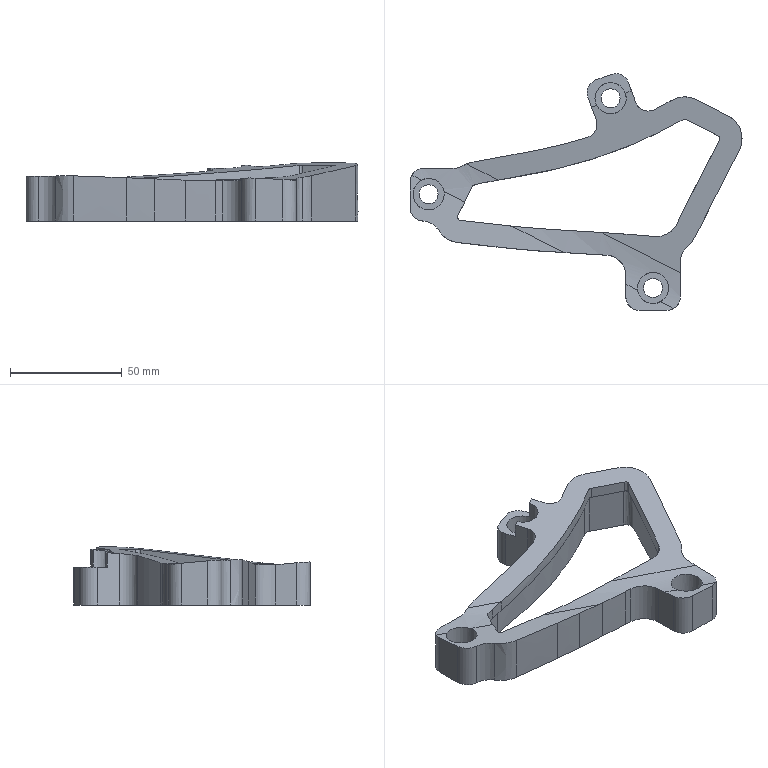Part | STEP file | gslz 2016.10.28-13_id358_x_t | 1 solid | 93 faces | box 148.689 x 106.005 x 26.001 mm | volume 75258 mm3 | other 35 | spline 26 | cylinder 18 | plane 14 | commonest cylinder face diameters 12 x8 18 x4 8.5 x3 14 x3